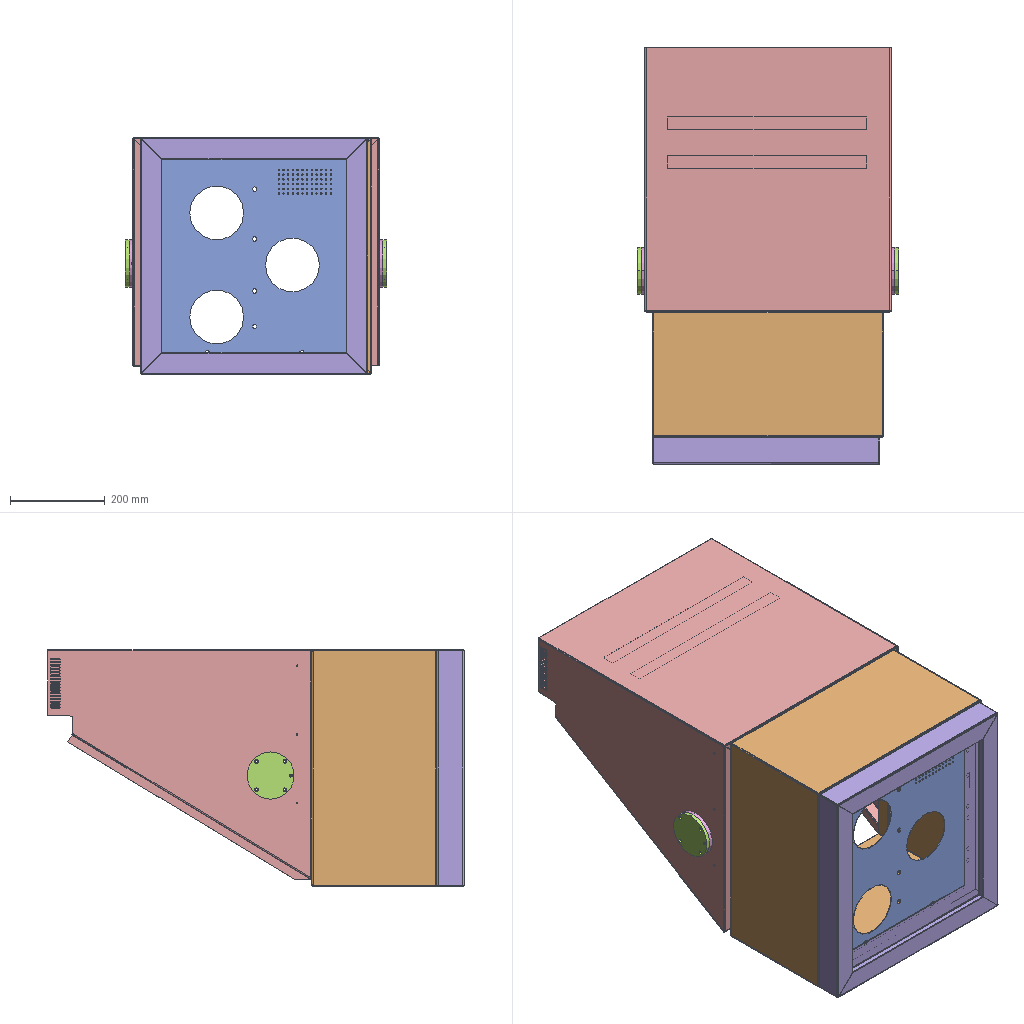Assembly | SolidWorks | 15 different items | 18 placed | box 552 x 880 x 500 mm
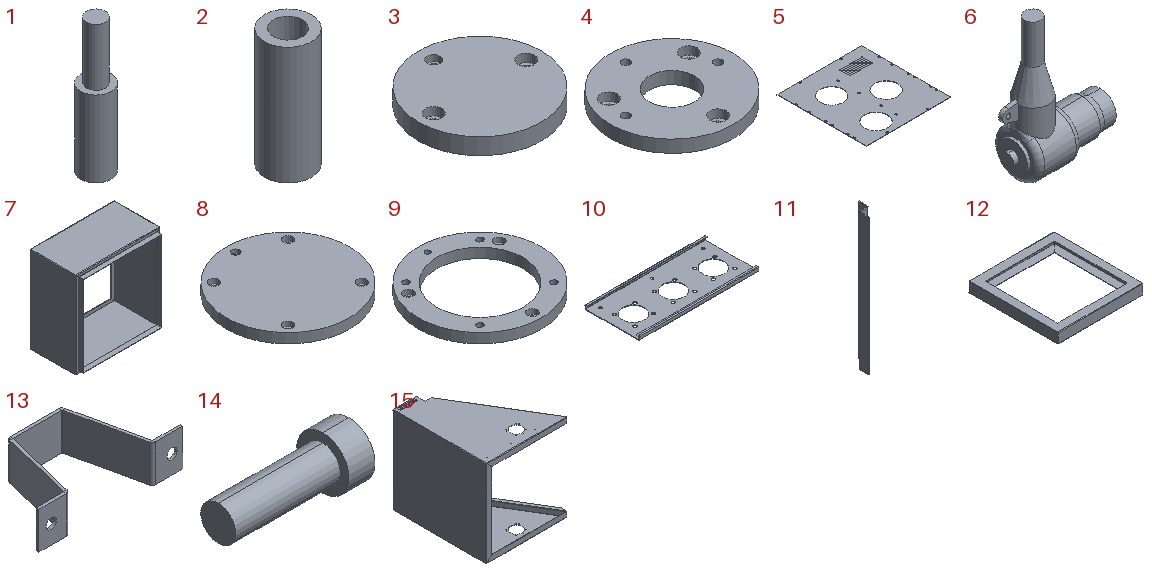Parts list (item | quantity | size | volume | features):
1 | x1 | 16 x 16 x 70 mm | 10399 mm3 | features Extrusion 1, ICE 1
2 | x1 | 16 x 16 x 40 mm | 5451 mm3 | features Extrusion 1, ICE 1
3 | x1 | 60 x 60 x 8 mm | 21900 mm3 | features ICE 2, FlatPattern 1, SMBaseFlange 1, SheetMetal 1
4 | x1 | 60 x 60 x 6 mm | 13737 mm3 | features FlatPattern 1, ICE 1, SMBaseFlange 1, SheetMetal 1
5 | x1 | 422 x 442 x 1.5 mm | 231306 mm3 | features FlatPattern 1, SMBaseFlange 1, SheetMetal 1
6 | x1 | 168.244 x 78.608 x 230.304 mm | 658696 mm3 | features ICE 6, Fillet 2, Revolution 1
7 | x1 | 488 x 290 x 500 mm | 1251248 mm3 | features EdgeFlange 3, SMMiteredFlange 2, FlatPattern 1, SMBaseFlange 1, SheetMetal 1
8 | x2 | 100 x 100 x 8 mm | 61554 mm3 | features ICE 4, Extrusion 1
9 | x2 | 100 x 100 x 8 mm | 30466 mm3 | features ICE 5, Extrusion 1
10 | x1 | 420 x 190 x 15 mm | 158753 mm3 | features EdgeFlange 4, FlatPattern 1, SMBaseFlange 1, SheetMetal 1
11 | x2 | 30 x 60 x 420 mm | 72668 mm3 | features FlatPattern 1, SMBaseFlange 1, SheetMetal 1
12 | x1 | 480 x 500 x 58 mm | 526033 mm3 | features FlatPattern 1, ICE 1, SMBaseFlange 1, SMMiteredFlange 1, SheetMetal 1
13 | x1 | 155 x 83 x 40 mm | 33033 mm3 | features FlatPattern 1, ICE 1, SMBaseFlange 1, SheetMetal 1
14 | x1 | 15 x 6 x 6 mm | 235.619 mm3 | features Revolution 1
15 | x1 | 485.154 x 558 x 520 mm | 1443065 mm3 | features EdgeFlange 6, ICE 6, FlatPattern 1, SMBaseFlange 1, SMMiteredFlange 1, SheetMetal 1
Mates (type | each side: item.copy, entity, surface, feature):
Coincident | 9.1 face plane Boss-Extrude1 | 8.1 face plane Boss-Extrude1
Concentric | 8.1 face cylinder Boss-Extrude1 | 9.1 face cylinder Boss-Extrude1
Concentric | 8.1 face cylinder Cut-Extrude3 | 9.1 face cylinder Cut-Extrude1
Coincident | 15.1 face plane Edge-Flange4 | 9.1 face plane Boss-Extrude1
Concentric | 15.1 face cylinder Cut-Extrude3 | 9.1 face cylinder Boss-Extrude1
Coincident | 9.2 face plane Boss-Extrude1 | 8.2 face plane Boss-Extrude1
Concentric | 9.2 face cylinder Boss-Extrude1 | 8.2 face cylinder Boss-Extrude1
Coincident | 15.1 face plane Base-Flange1 | 9.2 face plane Boss-Extrude1
Concentric | 15.1 face cylinder Base-Flange1 | 9.2 face cylinder Boss-Extrude1
Concentric | 9.2 face cylinder Cut-Extrude1 | 8.2 face cylinder Cut-Extrude3
Concentric | 9.1 face cylinder Cut-Extrude2 | 8.2 face cylinder Cut-Extrude3
Concentric | 15.1 face cylinder Base-Flange1 | 8.1 face cylinder Cut-Extrude2
Coincident | 15.1 face plane Edge-Flange1 | 11.1 face plane Base-Flange1
DistanceDim | 15.1 face plane Edge-Flange4 | 11.1 edge
DistanceDim | 11.1 face plane Base-Flange1 | 15.1 face plane Miter-Flange19
Coincident | 11.1 face plane Base-Flange1 | 11.2 face plane Base-Flange1 | 2 times
Coincident | 15.1 face plane Miter-Flange19 | 7.1 face plane Miter-Flange4 | 2 times
Coincident | 15.1 face plane Edge-Flange1 | 7.1 face plane Base-Flange1
Coincident | 5.1 face plane Base-Flange1 | 12.1 face plane Base-Flange1
DistanceDim | 5.1 face plane Base-Flange1 | 12.1 face plane Miter-Flange1 | 2 times
Coincident | 7.1 face plane Miter-Flange3 | 12.1 face plane Base-Flange1
Coincident | 7.1 face plane Edge-Flange1 | 12.1 face plane Miter-Flange1
Coincident | 7.1 face plane Base-Flange1 | 12.1 face plane Miter-Flange1
Coincident | 11.2 face plane Base-Flange1 | 10.1 face plane Edge-Flange2
Coincident | 11.2 face plane Base-Flange1 | 10.1 face plane Base-Flange1
Coincident | 11.1 face plane Base-Flange1 | 10.1 face plane Edge-Flange4
Coincident | 11.1 face plane Base-Flange1 | 10.1 face plane Base-Flange1